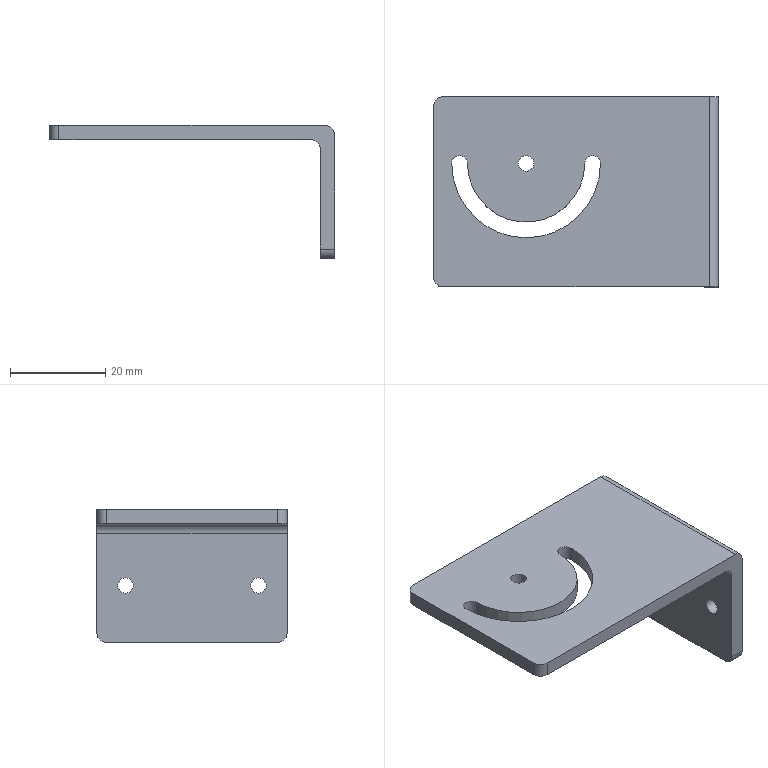Part | STEP file | SynoNew-0304-046 | 1 solid | 21 faces | box 60 x 40 x 28 mm | volume 9653 mm3 | cylinder 13 | plane 8 | commonest cylinder face diameters 4 x6 3.3 x3 3.242 x2 24.7 x1 31.3 x1
STEP:
#1=CARTESIAN_POINT('',(27.,14.,-11.379));
#2=VERTEX_POINT('',#1);
#3=CARTESIAN_POINT('',(27.,14.,-14.621));
#4=VERTEX_POINT('',#3);
#5=CARTESIAN_POINT('',(27.,14.,-13.));
#6=DIRECTION('',(1.,0.,0.));
#7=DIRECTION('',(0.,0.,1.));
#8=AXIS2_PLACEMENT_3D('',#5,#6,#7);
#9=CIRCLE('',#8,1.621);
#10=EDGE_CURVE('',#2,#4,#9,.T.);
#11=ORIENTED_EDGE('',*,*,#10,.F.);
#12=CARTESIAN_POINT('',(27.,14.,-13.));
#13=DIRECTION('',(1.,0.,0.));
#14=DIRECTION('',(0.,0.,1.));
#15=AXIS2_PLACEMENT_3D('',#12,#13,#14);
#16=CIRCLE('',#15,1.621);
#17=EDGE_CURVE('',#4,#2,#16,.T.);
#18=ORIENTED_EDGE('',*,*,#17,.F.);
#19=CARTESIAN_POINT('',(30.,14.,-14.621));
#20=VERTEX_POINT('',#19);
#21=CARTESIAN_POINT('',(104.356,14.,-14.621));
#22=DIRECTION('',(1.,0.,0.));
#23=VECTOR('',#22,1.621);
#24=LINE('',#21,#23);
#25=EDGE_CURVE('',#4,#20,#24,.T.);
#26=ORIENTED_EDGE('',*,*,#25,.T.);
#27=CARTESIAN_POINT('',(30.,14.,-13.));
#28=DIRECTION('',(-1.,0.,0.));
#29=DIRECTION('',(0.,0.,1.));
#30=AXIS2_PLACEMENT_3D('',#27,#28,#29);
#31=CIRCLE('',#30,1.621);
#32=EDGE_CURVE('',#20,#20,#31,.T.);
#33=ORIENTED_EDGE('',*,*,#32,.F.);
#34=ORIENTED_EDGE('',*,*,#25,.F.);
#35=EDGE_LOOP('',(#11,#18,#26,#33,#34));
#36=FACE_OUTER_BOUND('',#35,.T.);
#37=CARTESIAN_POINT('',(104.356,14.,-13.));
#38=DIRECTION('',(-1.,0.,0.));
#39=DIRECTION('',(0.,0.,1.));
#40=AXIS2_PLACEMENT_3D('',#37,#38,#39);
#41=CYLINDRICAL_SURFACE('',#40,1.621);
#42=ADVANCED_FACE('',(#36),#41,.F.);
#43=CARTESIAN_POINT('',(27.,-14.,-11.379));
#44=VERTEX_POINT('',#43);
#45=CARTESIAN_POINT('',(27.,-14.,-14.621));
#46=VERTEX_POINT('',#45);
#47=CARTESIAN_POINT('',(27.,-14.,-13.));
#48=DIRECTION('',(1.,0.,0.));
#49=DIRECTION('',(0.,0.,1.));
#50=AXIS2_PLACEMENT_3D('',#47,#48,#49);
#51=CIRCLE('',#50,1.621);
#52=EDGE_CURVE('',#44,#46,#51,.T.);
#53=ORIENTED_EDGE('',*,*,#52,.F.);
#54=CARTESIAN_POINT('',(27.,-14.,-13.));
#55=DIRECTION('',(1.,0.,0.));
#56=DIRECTION('',(0.,0.,1.));
#57=AXIS2_PLACEMENT_3D('',#54,#55,#56);
#58=CIRCLE('',#57,1.621);
#59=EDGE_CURVE('',#46,#44,#58,.T.);
#60=ORIENTED_EDGE('',*,*,#59,.F.);
#61=CARTESIAN_POINT('',(30.,-14.,-14.621));
#62=VERTEX_POINT('',#61);
#63=CARTESIAN_POINT('',(104.356,-14.,-14.621));
#64=DIRECTION('',(1.,0.,0.));
#65=VECTOR('',#64,1.621);
#66=LINE('',#63,#65);
#67=EDGE_CURVE('',#46,#62,#66,.T.);
#68=ORIENTED_EDGE('',*,*,#67,.T.);
#69=CARTESIAN_POINT('',(30.,-14.,-13.));
#70=DIRECTION('',(-1.,0.,0.));
#71=DIRECTION('',(0.,0.,1.));
#72=AXIS2_PLACEMENT_3D('',#69,#70,#71);
#73=CIRCLE('',#72,1.621);
#74=EDGE_CURVE('',#62,#62,#73,.T.);
#75=ORIENTED_EDGE('',*,*,#74,.F.);
#76=ORIENTED_EDGE('',*,*,#67,.F.);
#77=EDGE_LOOP('',(#53,#60,#68,#75,#76));
#78=FACE_OUTER_BOUND('',#77,.T.);
#79=CARTESIAN_POINT('',(104.356,-14.,-13.));
#80=DIRECTION('',(-1.,0.,0.));
#81=DIRECTION('',(0.,0.,1.));
#82=AXIS2_PLACEMENT_3D('',#79,#80,#81);
#83=CYLINDRICAL_SURFACE('',#82,1.621);
#84=ADVANCED_FACE('',(#78),#83,.F.);
#85=CARTESIAN_POINT('',(27.,-20.,-23.));
#86=VERTEX_POINT('',#85);
#87=CARTESIAN_POINT('',(27.,-18.,-25.));
#88=VERTEX_POINT('',#87);
#89=CARTESIAN_POINT('',(27.,-18.,-23.));
#90=DIRECTION('',(1.,0.,0.));
#91=DIRECTION('',(0.,-0.7071,-0.7071));
#92=AXIS2_PLACEMENT_3D('',#89,#90,#91);
#93=CIRCLE('',#92,2.);
#94=EDGE_CURVE('',#86,#88,#93,.T.);
#95=ORIENTED_EDGE('',*,*,#94,.T.);
#96=CARTESIAN_POINT('',(30.,-18.,-25.));
#97=VERTEX_POINT('',#96);
#98=CARTESIAN_POINT('',(-0.75,-18.,-25.));
#99=DIRECTION('',(1.,0.,0.));
#100=VECTOR('',#99,10.);
#101=LINE('',#98,#100);
#102=EDGE_CURVE('',#88,#97,#101,.T.);
#103=ORIENTED_EDGE('',*,*,#102,.T.);
#104=CARTESIAN_POINT('',(30.,-20.,-23.));
#105=VERTEX_POINT('',#104);
#106=CARTESIAN_POINT('',(30.,-18.,-23.));
#107=DIRECTION('',(-1.,0.,0.));
#108=DIRECTION('',(0.,-0.7071,-0.7071));
#109=AXIS2_PLACEMENT_3D('',#106,#107,#108);
#110=CIRCLE('',#109,2.);
#111=EDGE_CURVE('',#97,#105,#110,.T.);
#112=ORIENTED_EDGE('',*,*,#111,.T.);
#113=CARTESIAN_POINT('',(-0.75,-20.,-23.));
#114=DIRECTION('',(-1.,0.,0.));
#115=VECTOR('',#114,10.);
#116=LINE('',#113,#115);
#117=EDGE_CURVE('',#105,#86,#116,.T.);
#118=ORIENTED_EDGE('',*,*,#117,.T.);
#119=EDGE_LOOP('',(#95,#103,#112,#118));
#120=FACE_OUTER_BOUND('',#119,.T.);
#121=CARTESIAN_POINT('',(-0.75,-18.,-23.));
#122=DIRECTION('',(-1.,0.,0.));
#123=DIRECTION('',(0.,-0.7071,-0.7071));
#124=AXIS2_PLACEMENT_3D('',#121,#122,#123);
#125=CYLINDRICAL_SURFACE('',#124,2.);
#126=ADVANCED_FACE('',(#120),#125,.T.);
#127=ORIENTED_EDGE('',*,*,#117,.F.);
#128=CARTESIAN_POINT('',(30.,-20.,1.));
#129=VERTEX_POINT('',#128);
#130=CARTESIAN_POINT('',(30.,-20.,0.));
#131=DIRECTION('',(0.,0.,1.));
#132=VECTOR('',#131,10.);
#133=LINE('',#130,#132);
#134=EDGE_CURVE('',#105,#129,#133,.T.);
#135=ORIENTED_EDGE('',*,*,#134,.T.);
#136=CARTESIAN_POINT('',(28.,-20.,3.));
#137=VERTEX_POINT('',#136);
#138=CARTESIAN_POINT('',(28.,-20.,1.));
#139=DIRECTION('',(0.,1.,0.));
#140=DIRECTION('',(0.7071,0.,0.7071));
#141=AXIS2_PLACEMENT_3D('',#138,#139,#140);
#142=CIRCLE('',#141,2.);
#143=EDGE_CURVE('',#137,#129,#142,.T.);
#144=ORIENTED_EDGE('',*,*,#143,.F.);
#145=CARTESIAN_POINT('',(-28.,-20.,3.));
#146=VERTEX_POINT('',#145);
#147=CARTESIAN_POINT('',(-30.,-20.,3.));
#148=DIRECTION('',(1.,0.,0.));
#149=VECTOR('',#148,10.);
#150=LINE('',#147,#149);
#151=EDGE_CURVE('',#146,#137,#150,.T.);
#152=ORIENTED_EDGE('',*,*,#151,.F.);
#153=CARTESIAN_POINT('',(-28.,-20.,0.));
#154=VERTEX_POINT('',#153);
#155=CARTESIAN_POINT('',(-28.,-20.,0.));
#156=DIRECTION('',(0.,0.,1.));
#157=VECTOR('',#156,10.);
#158=LINE('',#155,#157);
#159=EDGE_CURVE('',#154,#146,#158,.T.);
#160=ORIENTED_EDGE('',*,*,#159,.F.);
#161=CARTESIAN_POINT('',(25.,-20.,0.));
#162=VERTEX_POINT('',#161);
#163=CARTESIAN_POINT('',(-30.,-20.,0.));
#164=DIRECTION('',(1.,0.,0.));
#165=VECTOR('',#164,10.);
#166=LINE('',#163,#165);
#167=EDGE_CURVE('',#154,#162,#166,.T.);
#168=ORIENTED_EDGE('',*,*,#167,.T.);
#169=CARTESIAN_POINT('',(27.,-20.,-2.));
#170=VERTEX_POINT('',#169);
#171=CARTESIAN_POINT('',(25.,-20.,-2.));
#172=DIRECTION('',(0.,-1.,0.));
#173=DIRECTION('',(0.7071,0.,0.7071));
#174=AXIS2_PLACEMENT_3D('',#171,#172,#173);
#175=CIRCLE('',#174,2.);
#176=EDGE_CURVE('',#170,#162,#175,.T.);
#177=ORIENTED_EDGE('',*,*,#176,.F.);
#178=CARTESIAN_POINT('',(27.,-20.,0.));
#179=DIRECTION('',(0.,0.,-1.));
#180=VECTOR('',#179,10.);
#181=LINE('',#178,#180);
#182=EDGE_CURVE('',#170,#86,#181,.T.);
#183=ORIENTED_EDGE('',*,*,#182,.T.);
#184=EDGE_LOOP('',(#127,#135,#144,#152,#160,#168,#177,#183));
#185=FACE_OUTER_BOUND('',#184,.T.);
#186=CARTESIAN_POINT('',(-30.,-20.,0.));
#187=DIRECTION('',(0.,-1.,0.));
#188=DIRECTION('',(1.,0.,0.));
#189=AXIS2_PLACEMENT_3D('',#186,#187,#188);
#190=PLANE('',#189);
#191=ADVANCED_FACE('',(#185),#190,.T.);
#192=ORIENTED_EDGE('',*,*,#111,.F.);
#193=CARTESIAN_POINT('',(30.,18.,-25.));
#194=VERTEX_POINT('',#193);
#195=CARTESIAN_POINT('',(30.,20.,-25.));
#196=DIRECTION('',(0.,-1.,0.));
#197=VECTOR('',#196,10.);
#198=LINE('',#195,#197);
#199=EDGE_CURVE('',#194,#97,#198,.T.);
#200=ORIENTED_EDGE('',*,*,#199,.F.);
#201=CARTESIAN_POINT('',(30.,20.,-23.));
#202=VERTEX_POINT('',#201);
#203=CARTESIAN_POINT('',(30.,18.,-23.));
#204=DIRECTION('',(-1.,0.,0.));
#205=DIRECTION('',(0.,0.7071,-0.7071));
#206=AXIS2_PLACEMENT_3D('',#203,#204,#205);
#207=CIRCLE('',#206,2.);
#208=EDGE_CURVE('',#202,#194,#207,.T.);
#209=ORIENTED_EDGE('',*,*,#208,.F.);
#210=CARTESIAN_POINT('',(30.,20.,1.));
#211=VERTEX_POINT('',#210);
#212=CARTESIAN_POINT('',(30.,20.,0.));
#213=DIRECTION('',(0.,0.,1.));
#214=VECTOR('',#213,10.);
#215=LINE('',#212,#214);
#216=EDGE_CURVE('',#202,#211,#215,.T.);
#217=ORIENTED_EDGE('',*,*,#216,.T.);
#218=CARTESIAN_POINT('',(30.,-10.,1.));
#219=DIRECTION('',(0.,1.,0.));
#220=VECTOR('',#219,10.);
#221=LINE('',#218,#220);
#222=EDGE_CURVE('',#129,#211,#221,.T.);
#223=ORIENTED_EDGE('',*,*,#222,.F.);
#224=ORIENTED_EDGE('',*,*,#134,.F.);
#225=EDGE_LOOP('',(#192,#200,#209,#217,#223,#224));
#226=FACE_OUTER_BOUND('',#225,.T.);
#227=ORIENTED_EDGE('',*,*,#32,.T.);
#228=EDGE_LOOP('',(#227));
#229=FACE_BOUND('',#228,.T.);
#230=ORIENTED_EDGE('',*,*,#74,.T.);
#231=EDGE_LOOP('',(#230));
#232=FACE_BOUND('',#231,.T.);
#233=CARTESIAN_POINT('',(30.,-20.,0.));
#234=DIRECTION('',(1.,0.,0.));
#235=DIRECTION('',(0.,1.,0.));
#236=AXIS2_PLACEMENT_3D('',#233,#234,#235);
#237=PLANE('',#236);
#238=ADVANCED_FACE('',(#226,#229,#232),#237,.T.);
#239=ORIENTED_EDGE('',*,*,#208,.T.);
#240=CARTESIAN_POINT('',(27.,18.,-25.));
#241=VERTEX_POINT('',#240);
#242=CARTESIAN_POINT('',(29.25,18.,-25.));
#243=DIRECTION('',(-1.,0.,0.));
#244=VECTOR('',#243,10.);
#245=LINE('',#242,#244);
#246=EDGE_CURVE('',#194,#241,#245,.T.);
#247=ORIENTED_EDGE('',*,*,#246,.T.);
#248=CARTESIAN_POINT('',(27.,20.,-23.));
#249=VERTEX_POINT('',#248);
#250=CARTESIAN_POINT('',(27.,18.,-23.));
#251=DIRECTION('',(1.,0.,0.));
#252=DIRECTION('',(0.,0.7071,-0.7071));
#253=AXIS2_PLACEMENT_3D('',#250,#251,#252);
#254=CIRCLE('',#253,2.);
#255=EDGE_CURVE('',#241,#249,#254,.T.);
#256=ORIENTED_EDGE('',*,*,#255,.T.);
#257=CARTESIAN_POINT('',(29.25,20.,-23.));
#258=DIRECTION('',(1.,0.,0.));
#259=VECTOR('',#258,10.);
#260=LINE('',#257,#259);
#261=EDGE_CURVE('',#249,#202,#260,.T.);
#262=ORIENTED_EDGE('',*,*,#261,.T.);
#263=EDGE_LOOP('',(#239,#247,#256,#262));
#264=FACE_OUTER_BOUND('',#263,.T.);
#265=CARTESIAN_POINT('',(29.25,18.,-23.));
#266=DIRECTION('',(1.,0.,0.));
#267=DIRECTION('',(0.,0.7071,-0.7071));
#268=AXIS2_PLACEMENT_3D('',#265,#266,#267);
#269=CYLINDRICAL_SURFACE('',#268,2.);
#270=ADVANCED_FACE('',(#264),#269,.T.);
#271=ORIENTED_EDGE('',*,*,#261,.F.);
#272=CARTESIAN_POINT('',(27.,20.,-2.));
#273=VERTEX_POINT('',#272);
#274=CARTESIAN_POINT('',(27.,20.,0.));
#275=DIRECTION('',(0.,0.,-1.));
#276=VECTOR('',#275,10.);
#277=LINE('',#274,#276);
#278=EDGE_CURVE('',#273,#249,#277,.T.);
#279=ORIENTED_EDGE('',*,*,#278,.F.);
#280=CARTESIAN_POINT('',(25.,20.,0.));
#281=VERTEX_POINT('',#280);
#282=CARTESIAN_POINT('',(25.,20.,-2.));
#283=DIRECTION('',(0.,1.,0.));
#284=DIRECTION('',(0.7071,0.,0.7071));
#285=AXIS2_PLACEMENT_3D('',#282,#283,#284);
#286=CIRCLE('',#285,2.);
#287=EDGE_CURVE('',#281,#273,#286,.T.);
#288=ORIENTED_EDGE('',*,*,#287,.F.);
#289=CARTESIAN_POINT('',(-28.,20.,0.));
#290=VERTEX_POINT('',#289);
#291=CARTESIAN_POINT('',(30.,20.,0.));
#292=DIRECTION('',(-1.,0.,0.));
#293=VECTOR('',#292,10.);
#294=LINE('',#291,#293);
#295=EDGE_CURVE('',#281,#290,#294,.T.);
#296=ORIENTED_EDGE('',*,*,#295,.T.);
#297=CARTESIAN_POINT('',(-28.,20.,3.));
#298=VERTEX_POINT('',#297);
#299=CARTESIAN_POINT('',(-28.,20.,0.));
#300=DIRECTION('',(0.,0.,-1.));
#301=VECTOR('',#300,10.);
#302=LINE('',#299,#301);
#303=EDGE_CURVE('',#298,#290,#302,.T.);
#304=ORIENTED_EDGE('',*,*,#303,.F.);
#305=CARTESIAN_POINT('',(28.,20.,3.));
#306=VERTEX_POINT('',#305);
#307=CARTESIAN_POINT('',(30.,20.,3.));
#308=DIRECTION('',(-1.,0.,0.));
#309=VECTOR('',#308,10.);
#310=LINE('',#307,#309);
#311=EDGE_CURVE('',#306,#298,#310,.T.);
#312=ORIENTED_EDGE('',*,*,#311,.F.);
#313=CARTESIAN_POINT('',(28.,20.,1.));
#314=DIRECTION('',(0.,-1.,0.));
#315=DIRECTION('',(0.7071,0.,0.7071));
#316=AXIS2_PLACEMENT_3D('',#313,#314,#315);
#317=CIRCLE('',#316,2.);
#318=EDGE_CURVE('',#211,#306,#317,.T.);
#319=ORIENTED_EDGE('',*,*,#318,.F.);
#320=ORIENTED_EDGE('',*,*,#216,.F.);
#321=EDGE_LOOP('',(#271,#279,#288,#296,#304,#312,#319,#320));
#322=FACE_OUTER_BOUND('',#321,.T.);
#323=CARTESIAN_POINT('',(30.,20.,0.));
#324=DIRECTION('',(0.,1.,0.));
#325=DIRECTION('',(-1.,0.,0.));
#326=AXIS2_PLACEMENT_3D('',#323,#324,#325);
#327=PLANE('',#326);
#328=ADVANCED_FACE('',(#322),#327,.T.);
#329=CARTESIAN_POINT('',(-30.,-18.,3.));
#330=VERTEX_POINT('',#329);
#331=CARTESIAN_POINT('',(-28.,-18.,3.));
#332=DIRECTION('',(0.,0.,-1.));
#333=DIRECTION('',(-0.7071,-0.7071,0.));
#334=AXIS2_PLACEMENT_3D('',#331,#332,#333);
#335=CIRCLE('',#334,2.);
#336=EDGE_CURVE('',#146,#330,#335,.T.);
#337=ORIENTED_EDGE('',*,*,#336,.T.);
#338=CARTESIAN_POINT('',(-30.,-18.,0.));
#339=VERTEX_POINT('',#338);
#340=CARTESIAN_POINT('',(-30.,-18.,0.));
#341=DIRECTION('',(0.,0.,-1.));
#342=VECTOR('',#341,10.);
#343=LINE('',#340,#342);
#344=EDGE_CURVE('',#330,#339,#343,.T.);
#345=ORIENTED_EDGE('',*,*,#344,.T.);
#346=CARTESIAN_POINT('',(-28.,-18.,0.));
#347=DIRECTION('',(0.,0.,1.));
#348=DIRECTION('',(-0.7071,-0.7071,0.));
#349=AXIS2_PLACEMENT_3D('',#346,#347,#348);
#350=CIRCLE('',#349,2.);
#351=EDGE_CURVE('',#339,#154,#350,.T.);
#352=ORIENTED_EDGE('',*,*,#351,.T.);
#353=ORIENTED_EDGE('',*,*,#159,.T.);
#354=EDGE_LOOP('',(#337,#345,#352,#353));
#355=FACE_OUTER_BOUND('',#354,.T.);
#356=CARTESIAN_POINT('',(-28.,-18.,0.));
#357=DIRECTION('',(0.,0.,1.));
#358=DIRECTION('',(-0.7071,-0.7071,0.));
#359=AXIS2_PLACEMENT_3D('',#356,#357,#358);
#360=CYLINDRICAL_SURFACE('',#359,2.);
#361=ADVANCED_FACE('',(#355),#360,.T.);
#362=ORIENTED_EDGE('',*,*,#351,.F.);
#363=CARTESIAN_POINT('',(-30.,18.,0.));
#364=VERTEX_POINT('',#363);
#365=CARTESIAN_POINT('',(-30.,20.,0.));
#366=DIRECTION('',(0.,-1.,0.));
#367=VECTOR('',#366,10.);
#368=LINE('',#365,#367);
#369=EDGE_CURVE('',#364,#339,#368,.T.);
#370=ORIENTED_EDGE('',*,*,#369,.F.);
#371=CARTESIAN_POINT('',(-28.,18.,0.));
#372=DIRECTION('',(0.,0.,1.));
#373=DIRECTION('',(-0.7071,0.7071,0.));
#374=AXIS2_PLACEMENT_3D('',#371,#372,#373);
#375=CIRCLE('',#374,2.);
#376=EDGE_CURVE('',#290,#364,#375,.T.);
#377=ORIENTED_EDGE('',*,*,#376,.F.);
#378=ORIENTED_EDGE('',*,*,#295,.F.);
#379=CARTESIAN_POINT('',(25.,-10.,0.));
#380=DIRECTION('',(0.,1.,0.));
#381=VECTOR('',#380,10.);
#382=LINE('',#379,#381);
#383=EDGE_CURVE('',#162,#281,#382,.T.);
#384=ORIENTED_EDGE('',*,*,#383,.F.);
#385=ORIENTED_EDGE('',*,*,#167,.F.);
#386=EDGE_LOOP('',(#362,#370,#377,#378,#384,#385));
#387=FACE_OUTER_BOUND('',#386,.T.);
#388=CARTESIAN_POINT('',(-8.85,6.,0.));
#389=VERTEX_POINT('',#388);
#390=CARTESIAN_POINT('',(-12.15,6.,0.));
#391=VERTEX_POINT('',#390);
#392=CARTESIAN_POINT('',(-10.5,6.,0.));
#393=DIRECTION('',(0.,0.,1.));
#394=DIRECTION('',(1.,0.,0.));
#395=AXIS2_PLACEMENT_3D('',#392,#393,#394);
#396=CIRCLE('',#395,1.65);
#397=EDGE_CURVE('',#389,#391,#396,.T.);
#398=ORIENTED_EDGE('',*,*,#397,.T.);
#399=CARTESIAN_POINT('',(-10.5,6.,0.));
#400=DIRECTION('',(0.,0.,1.));
#401=DIRECTION('',(1.,0.,0.));
#402=AXIS2_PLACEMENT_3D('',#399,#400,#401);
#403=CIRCLE('',#402,1.65);
#404=EDGE_CURVE('',#391,#389,#403,.T.);
#405=ORIENTED_EDGE('',*,*,#404,.T.);
#406=EDGE_LOOP('',(#398,#405));
#407=FACE_BOUND('',#406,.T.);
#408=CARTESIAN_POINT('',(5.15,6.,0.));
#409=VERTEX_POINT('',#408);
#410=CARTESIAN_POINT('',(1.85,6.,0.));
#411=VERTEX_POINT('',#410);
#412=CARTESIAN_POINT('',(3.5,6.,0.));
#413=DIRECTION('',(0.,0.,1.));
#414=DIRECTION('',(1.,0.,0.));
#415=AXIS2_PLACEMENT_3D('',#412,#413,#414);
#416=CIRCLE('',#415,1.65);
#417=EDGE_CURVE('',#409,#411,#416,.T.);
#418=ORIENTED_EDGE('',*,*,#417,.T.);
#419=CARTESIAN_POINT('',(-22.85,6.,0.));
#420=VERTEX_POINT('',#419);
#421=CARTESIAN_POINT('',(-10.5,6.,0.));
#422=DIRECTION('',(0.,0.,-1.));
#423=DIRECTION('',(1.,0.,0.));
#424=AXIS2_PLACEMENT_3D('',#421,#422,#423);
#425=CIRCLE('',#424,12.35);
#426=EDGE_CURVE('',#411,#420,#425,.T.);
#427=ORIENTED_EDGE('',*,*,#426,.T.);
#428=CARTESIAN_POINT('',(-26.15,6.,0.));
#429=VERTEX_POINT('',#428);
#430=CARTESIAN_POINT('',(-24.5,6.,0.));
#431=DIRECTION('',(0.,0.,1.));
#432=DIRECTION('',(1.,0.,0.));
#433=AXIS2_PLACEMENT_3D('',#430,#431,#432);
#434=CIRCLE('',#433,1.65);
#435=EDGE_CURVE('',#420,#429,#434,.T.);
#436=ORIENTED_EDGE('',*,*,#435,.T.);
#437=CARTESIAN_POINT('',(-10.5,6.,0.));
#438=DIRECTION('',(0.,0.,1.));
#439=DIRECTION('',(-1.,0.,0.));
#440=AXIS2_PLACEMENT_3D('',#437,#438,#439);
#441=CIRCLE('',#440,15.65);
#442=EDGE_CURVE('',#429,#409,#441,.T.);
#443=ORIENTED_EDGE('',*,*,#442,.T.);
#444=EDGE_LOOP('',(#418,#427,#436,#443));
#445=FACE_BOUND('',#444,.T.);
#446=CARTESIAN_POINT('',(0.,0.,0.));
#447=DIRECTION('',(0.,0.,1.));
#448=DIRECTION('',(1.,0.,0.));
#449=AXIS2_PLACEMENT_3D('',#446,#447,#448);
#450=PLANE('',#449);
#451=ADVANCED_FACE('',(#387,#407,#445),#450,.F.);
#452=CARTESIAN_POINT('',(-30.,18.,3.));
#453=VERTEX_POINT('',#452);
#454=CARTESIAN_POINT('',(-28.,18.,3.));
#455=DIRECTION('',(0.,0.,-1.));
#456=DIRECTION('',(-0.7071,0.7071,0.));
#457=AXIS2_PLACEMENT_3D('',#454,#455,#456);
#458=CIRCLE('',#457,2.);
#459=EDGE_CURVE('',#453,#298,#458,.T.);
#460=ORIENTED_EDGE('',*,*,#459,.T.);
#461=ORIENTED_EDGE('',*,*,#303,.T.);
#462=ORIENTED_EDGE('',*,*,#376,.T.);
#463=CARTESIAN_POINT('',(-30.,18.,0.));
#464=DIRECTION('',(0.,0.,1.));
#465=VECTOR('',#464,10.);
#466=LINE('',#463,#465);
#467=EDGE_CURVE('',#364,#453,#466,.T.);
#468=ORIENTED_EDGE('',*,*,#467,.T.);
#469=EDGE_LOOP('',(#460,#461,#462,#468));
#470=FACE_OUTER_BOUND('',#469,.T.);
#471=CARTESIAN_POINT('',(-28.,18.,0.));
#472=DIRECTION('',(0.,0.,1.));
#473=DIRECTION('',(-0.7071,0.7071,0.));
#474=AXIS2_PLACEMENT_3D('',#471,#472,#473);
#475=CYLINDRICAL_SURFACE('',#474,2.);
#476=ADVANCED_FACE('',(#470),#475,.T.);
#477=ORIENTED_EDGE('',*,*,#336,.F.);
#478=ORIENTED_EDGE('',*,*,#151,.T.);
#479=CARTESIAN_POINT('',(28.,-10.,3.));
#480=DIRECTION('',(0.,-1.,0.));
#481=VECTOR('',#480,10.);
#482=LINE('',#479,#481);
#483=EDGE_CURVE('',#306,#137,#482,.T.);
#484=ORIENTED_EDGE('',*,*,#483,.F.);
#485=ORIENTED_EDGE('',*,*,#311,.T.);
#486=ORIENTED_EDGE('',*,*,#459,.F.);
#487=CARTESIAN_POINT('',(-30.,20.,3.));
#488=DIRECTION('',(0.,-1.,0.));
#489=VECTOR('',#488,10.);
#490=LINE('',#487,#489);
#491=EDGE_CURVE('',#453,#330,#490,.T.);
#492=ORIENTED_EDGE('',*,*,#491,.T.);
#493=EDGE_LOOP('',(#477,#478,#484,#485,#486,#492));
#494=FACE_OUTER_BOUND('',#493,.T.);
#495=CARTESIAN_POINT('',(-8.85,6.,3.));
#496=VERTEX_POINT('',#495);
#497=CARTESIAN_POINT('',(-12.15,6.,3.));
#498=VERTEX_POINT('',#497);
#499=CARTESIAN_POINT('',(-10.5,6.,3.));
#500=DIRECTION('',(0.,0.,-1.));
#501=DIRECTION('',(1.,0.,0.));
#502=AXIS2_PLACEMENT_3D('',#499,#500,#501);
#503=CIRCLE('',#502,1.65);
#504=EDGE_CURVE('',#496,#498,#503,.T.);
#505=ORIENTED_EDGE('',*,*,#504,.T.);
#506=CARTESIAN_POINT('',(-10.5,6.,3.));
#507=DIRECTION('',(0.,0.,-1.));
#508=DIRECTION('',(1.,0.,0.));
#509=AXIS2_PLACEMENT_3D('',#506,#507,#508);
#510=CIRCLE('',#509,1.65);
#511=EDGE_CURVE('',#498,#496,#510,.T.);
#512=ORIENTED_EDGE('',*,*,#511,.T.);
#513=EDGE_LOOP('',(#505,#512));
#514=FACE_BOUND('',#513,.T.);
#515=CARTESIAN_POINT('',(1.85,6.,3.));
#516=VERTEX_POINT('',#515);
#517=CARTESIAN_POINT('',(5.15,6.,3.));
#518=VERTEX_POINT('',#517);
#519=CARTESIAN_POINT('',(3.5,6.,3.));
#520=DIRECTION('',(0.,0.,-1.));
#521=DIRECTION('',(1.,0.,0.));
#522=AXIS2_PLACEMENT_3D('',#519,#520,#521);
#523=CIRCLE('',#522,1.65);
#524=EDGE_CURVE('',#516,#518,#523,.T.);
#525=ORIENTED_EDGE('',*,*,#524,.T.);
#526=CARTESIAN_POINT('',(-26.15,6.,3.));
#527=VERTEX_POINT('',#526);
#528=CARTESIAN_POINT('',(-10.5,6.,3.));
#529=DIRECTION('',(0.,0.,-1.));
#530=DIRECTION('',(-1.,0.,0.));
#531=AXIS2_PLACEMENT_3D('',#528,#529,#530);
#532=CIRCLE('',#531,15.65);
#533=EDGE_CURVE('',#518,#527,#532,.T.);
#534=ORIENTED_EDGE('',*,*,#533,.T.);
#535=CARTESIAN_POINT('',(-22.85,6.,3.));
#536=VERTEX_POINT('',#535);
#537=CARTESIAN_POINT('',(-24.5,6.,3.));
#538=DIRECTION('',(0.,0.,-1.));
#539=DIRECTION('',(1.,0.,0.));
#540=AXIS2_PLACEMENT_3D('',#537,#538,#539);
#541=CIRCLE('',#540,1.65);
#542=EDGE_CURVE('',#527,#536,#541,.T.);
#543=ORIENTED_EDGE('',*,*,#542,.T.);
#544=CARTESIAN_POINT('',(-10.5,6.,3.));
#545=DIRECTION('',(0.,0.,1.));
#546=DIRECTION('',(1.,0.,0.));
#547=AXIS2_PLACEMENT_3D('',#544,#545,#546);
#548=CIRCLE('',#547,12.35);
#549=EDGE_CURVE('',#536,#516,#548,.T.);
#550=ORIENTED_EDGE('',*,*,#549,.T.);
#551=EDGE_LOOP('',(#525,#534,#543,#550));
#552=FACE_BOUND('',#551,.T.);
#553=CARTESIAN_POINT('',(0.,0.,3.));
#554=DIRECTION('',(0.,0.,1.));
#555=DIRECTION('',(1.,0.,0.));
#556=AXIS2_PLACEMENT_3D('',#553,#554,#555);
#557=PLANE('',#556);
#558=ADVANCED_FACE('',(#494,#514,#552),#557,.T.);
#559=ORIENTED_EDGE('',*,*,#318,.T.);
#560=ORIENTED_EDGE('',*,*,#483,.T.);
#561=ORIENTED_EDGE('',*,*,#143,.T.);
#562=ORIENTED_EDGE('',*,*,#222,.T.);
#563=EDGE_LOOP('',(#559,#560,#561,#562));
#564=FACE_OUTER_BOUND('',#563,.T.);
#565=CARTESIAN_POINT('',(28.,-10.,1.));
#566=DIRECTION('',(0.,1.,0.));
#567=DIRECTION('',(0.7071,0.,0.7071));
#568=AXIS2_PLACEMENT_3D('',#565,#566,#567);
#569=CYLINDRICAL_SURFACE('',#568,2.);
#570=ADVANCED_FACE('',(#564),#569,.T.);
#571=ORIENTED_EDGE('',*,*,#287,.T.);
#572=CARTESIAN_POINT('',(27.,-10.,-2.));
#573=DIRECTION('',(0.,-1.,0.));
#574=VECTOR('',#573,10.);
#575=LINE('',#572,#574);
#576=EDGE_CURVE('',#273,#170,#575,.T.);
#577=ORIENTED_EDGE('',*,*,#576,.T.);
#578=ORIENTED_EDGE('',*,*,#176,.T.);
#579=ORIENTED_EDGE('',*,*,#383,.T.);
#580=EDGE_LOOP('',(#571,#577,#578,#579));
#581=FACE_OUTER_BOUND('',#580,.T.);
#582=CARTESIAN_POINT('',(25.,-10.,-2.));
#583=DIRECTION('',(0.,-1.,0.));
#584=DIRECTION('',(0.7071,0.,0.7071));
#585=AXIS2_PLACEMENT_3D('',#582,#583,#584);
#586=CYLINDRICAL_SURFACE('',#585,2.);
#587=ADVANCED_FACE('',(#581),#586,.F.);
#588=ORIENTED_EDGE('',*,*,#94,.F.);
#589=ORIENTED_EDGE('',*,*,#182,.F.);
#590=ORIENTED_EDGE('',*,*,#576,.F.);
#591=ORIENTED_EDGE('',*,*,#278,.T.);
#592=ORIENTED_EDGE('',*,*,#255,.F.);
#593=CARTESIAN_POINT('',(27.,-20.,-25.));
#594=DIRECTION('',(0.,1.,0.));
#595=VECTOR('',#594,10.);
#596=LINE('',#593,#595);
#597=EDGE_CURVE('',#88,#241,#596,.T.);
#598=ORIENTED_EDGE('',*,*,#597,.F.);
#599=EDGE_LOOP('',(#588,#589,#590,#591,#592,#598));
#600=FACE_OUTER_BOUND('',#599,.T.);
#601=ORIENTED_EDGE('',*,*,#10,.T.);
#602=ORIENTED_EDGE('',*,*,#17,.T.);
#603=EDGE_LOOP('',(#601,#602));
#604=FACE_BOUND('',#603,.T.);
#605=ORIENTED_EDGE('',*,*,#52,.T.);
#606=ORIENTED_EDGE('',*,*,#59,.T.);
#607=EDGE_LOOP('',(#605,#606));
#608=FACE_BOUND('',#607,.T.);
#609=CARTESIAN_POINT('',(27.,-20.,0.));
#610=DIRECTION('',(-1.,0.,0.));
#611=DIRECTION('',(0.,1.,0.));
#612=AXIS2_PLACEMENT_3D('',#609,#610,#611);
#613=PLANE('',#612);
#614=ADVANCED_FACE('',(#600,#604,#608),#613,.T.);
#615=ORIENTED_EDGE('',*,*,#102,.F.);
#616=ORIENTED_EDGE('',*,*,#597,.T.);
#617=ORIENTED_EDGE('',*,*,#246,.F.);
#618=ORIENTED_EDGE('',*,*,#199,.T.);
#619=EDGE_LOOP('',(#615,#616,#617,#618));
#620=FACE_OUTER_BOUND('',#619,.T.);
#621=CARTESIAN_POINT('',(28.5,0.,-25.));
#622=DIRECTION('',(0.,0.,-1.));
#623=DIRECTION('',(-1.,0.,0.));
#624=AXIS2_PLACEMENT_3D('',#621,#622,#623);
#625=PLANE('',#624);
#626=ADVANCED_FACE('',(#620),#625,.T.);
#627=ORIENTED_EDGE('',*,*,#504,.F.);
#628=ORIENTED_EDGE('',*,*,#511,.F.);
#629=CARTESIAN_POINT('',(-12.15,6.,3.));
#630=DIRECTION('',(0.,0.,-1.));
#631=VECTOR('',#630,1.65);
#632=LINE('',#629,#631);
#633=EDGE_CURVE('',#498,#391,#632,.T.);
#634=ORIENTED_EDGE('',*,*,#633,.T.);
#635=ORIENTED_EDGE('',*,*,#397,.F.);
#636=ORIENTED_EDGE('',*,*,#404,.F.);
#637=ORIENTED_EDGE('',*,*,#633,.F.);
#638=EDGE_LOOP('',(#627,#628,#634,#635,#636,#637));
#639=FACE_OUTER_BOUND('',#638,.T.);
#640=CARTESIAN_POINT('',(-10.5,6.,3.));
#641=DIRECTION('',(0.,0.,-1.));
#642=DIRECTION('',(1.,0.,0.));
#643=AXIS2_PLACEMENT_3D('',#640,#641,#642);
#644=CYLINDRICAL_SURFACE('',#643,1.65);
#645=ADVANCED_FACE('',(#639),#644,.F.);
#646=ORIENTED_EDGE('',*,*,#435,.F.);
#647=CARTESIAN_POINT('',(-22.85,6.,3.));
#648=DIRECTION('',(0.,0.,-1.));
#649=VECTOR('',#648,10.);
#650=LINE('',#647,#649);
#651=EDGE_CURVE('',#536,#420,#650,.T.);
#652=ORIENTED_EDGE('',*,*,#651,.F.);
#653=ORIENTED_EDGE('',*,*,#542,.F.);
#654=CARTESIAN_POINT('',(-26.15,6.,3.));
#655=DIRECTION('',(0.,0.,-1.));
#656=VECTOR('',#655,10.);
#657=LINE('',#654,#656);
#658=EDGE_CURVE('',#527,#429,#657,.T.);
#659=ORIENTED_EDGE('',*,*,#658,.T.);
#660=EDGE_LOOP('',(#646,#652,#653,#659));
#661=FACE_OUTER_BOUND('',#660,.T.);
#662=CARTESIAN_POINT('',(-24.5,6.,3.));
#663=DIRECTION('',(0.,0.,-1.));
#664=DIRECTION('',(1.,0.,0.));
#665=AXIS2_PLACEMENT_3D('',#662,#663,#664);
#666=CYLINDRICAL_SURFACE('',#665,1.65);
#667=ADVANCED_FACE('',(#661),#666,.F.);
#668=ORIENTED_EDGE('',*,*,#442,.F.);
#669=ORIENTED_EDGE('',*,*,#658,.F.);
#670=ORIENTED_EDGE('',*,*,#533,.F.);
#671=CARTESIAN_POINT('',(5.15,6.,3.));
#672=DIRECTION('',(0.,0.,-1.));
#673=VECTOR('',#672,10.);
#674=LINE('',#671,#673);
#675=EDGE_CURVE('',#518,#409,#674,.T.);
#676=ORIENTED_EDGE('',*,*,#675,.T.);
#677=EDGE_LOOP('',(#668,#669,#670,#676));
#678=FACE_OUTER_BOUND('',#677,.T.);
#679=CARTESIAN_POINT('',(-10.5,6.,3.));
#680=DIRECTION('',(0.,0.,-1.));
#681=DIRECTION('',(-1.,0.,0.));
#682=AXIS2_PLACEMENT_3D('',#679,#680,#681);
#683=CYLINDRICAL_SURFACE('',#682,15.65);
#684=ADVANCED_FACE('',(#678),#683,.F.);
#685=ORIENTED_EDGE('',*,*,#417,.F.);
#686=ORIENTED_EDGE('',*,*,#675,.F.);
#687=ORIENTED_EDGE('',*,*,#524,.F.);
#688=CARTESIAN_POINT('',(1.85,6.,3.));
#689=DIRECTION('',(0.,0.,-1.));
#690=VECTOR('',#689,10.);
#691=LINE('',#688,#690);
#692=EDGE_CURVE('',#516,#411,#691,.T.);
#693=ORIENTED_EDGE('',*,*,#692,.T.);
#694=EDGE_LOOP('',(#685,#686,#687,#693));
#695=FACE_OUTER_BOUND('',#694,.T.);
#696=CARTESIAN_POINT('',(3.5,6.,3.));
#697=DIRECTION('',(0.,0.,-1.));
#698=DIRECTION('',(1.,0.,0.));
#699=AXIS2_PLACEMENT_3D('',#696,#697,#698);
#700=CYLINDRICAL_SURFACE('',#699,1.65);
#701=ADVANCED_FACE('',(#695),#700,.F.);
#702=ORIENTED_EDGE('',*,*,#426,.F.);
#703=ORIENTED_EDGE('',*,*,#692,.F.);
#704=ORIENTED_EDGE('',*,*,#549,.F.);
#705=ORIENTED_EDGE('',*,*,#651,.T.);
#706=EDGE_LOOP('',(#702,#703,#704,#705));
#707=FACE_OUTER_BOUND('',#706,.T.);
#708=CARTESIAN_POINT('',(-10.5,6.,3.));
#709=DIRECTION('',(0.,0.,-1.));
#710=DIRECTION('',(1.,0.,0.));
#711=AXIS2_PLACEMENT_3D('',#708,#709,#710);
#712=CYLINDRICAL_SURFACE('',#711,12.35);
#713=ADVANCED_FACE('',(#707),#712,.T.);
#714=ORIENTED_EDGE('',*,*,#344,.F.);
#715=ORIENTED_EDGE('',*,*,#491,.F.);
#716=ORIENTED_EDGE('',*,*,#467,.F.);
#717=ORIENTED_EDGE('',*,*,#369,.T.);
#718=EDGE_LOOP('',(#714,#715,#716,#717));
#719=FACE_OUTER_BOUND('',#718,.T.);
#720=CARTESIAN_POINT('',(-30.,20.,0.));
#721=DIRECTION('',(-1.,0.,0.));
#722=DIRECTION('',(0.,-1.,0.));
#723=AXIS2_PLACEMENT_3D('',#720,#721,#722);
#724=PLANE('',#723);
#725=ADVANCED_FACE('',(#719),#724,.T.);
#726=CLOSED_SHELL('',(#42,#84,#126,#191,#238,#270,#328,#361,#451,#476,#558,#570,#587,#614,#626,#645,#667,#684,#701,#713,#725));
#727=MANIFOLD_SOLID_BREP('',#726);
#728=(LENGTH_UNIT()NAMED_UNIT(*)SI_UNIT(.MILLI.,.METRE.));
#729=UNCERTAINTY_MEASURE_WITH_UNIT(LENGTH_MEASURE(0.01),#728,'','');
#730=(NAMED_UNIT(*)PLANE_ANGLE_UNIT()SI_UNIT($,.RADIAN.));
#731=(NAMED_UNIT(*)SI_UNIT($,.STERADIAN.)SOLID_ANGLE_UNIT());
#732=(GEOMETRIC_REPRESENTATION_CONTEXT(3)GLOBAL_UNCERTAINTY_ASSIGNED_CONTEXT((#729))GLOBAL_UNIT_ASSIGNED_CONTEXT((#728,#730,#731))REPRESENTATION_CONTEXT('',''));
#733=ADVANCED_BREP_SHAPE_REPRESENTATION('',(#727),#732);